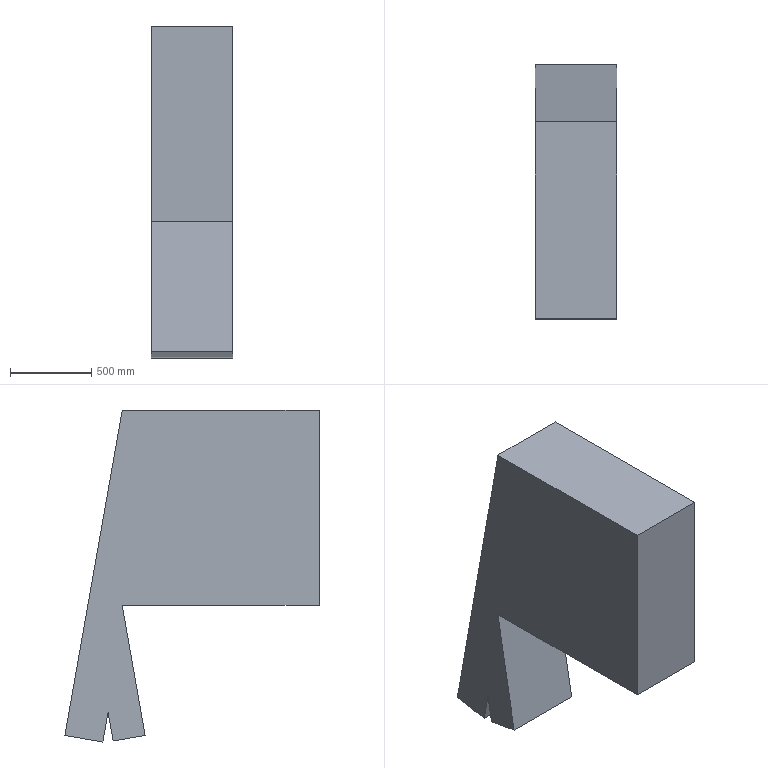Part | STEP file | Material rack | 1 solid | 11 faces | box 500 x 1564 x 2041 mm | volume 933674835 mm3 | plane 11
STEP:
#1=CARTESIAN_POINT('',(0.,0.,0.));
#2=DIRECTION('',(0.,0.,1.));
#3=DIRECTION('',(1.,0.,0.));
#4=AXIS2_PLACEMENT_3D('',#1,#2,#3);
#5=CARTESIAN_POINT('',(250.,1563.716,-800.));
#6=VERTEX_POINT('',#5);
#7=CARTESIAN_POINT('',(250.,1211.062,1200.));
#8=VERTEX_POINT('',#7);
#9=CARTESIAN_POINT('',(250.,1563.716,-800.));
#10=DIRECTION('',(0.,-0.1736,0.9848));
#11=VECTOR('',#10,1.);
#12=LINE('',#9,#11);
#13=CARTESIAN_POINT('',(250.,0.,0.));
#14=DIRECTION('',(1.,0.,0.));
#15=DIRECTION('',(0.,0.,-1.));
#16=AXIS2_PLACEMENT_3D('',#13,#14,#15);
#17=PLANE('',#16);
#18=CARTESIAN_POINT('',(800.,1563.716));
#19=DIRECTION('',(-0.9848,-0.1736));
#20=VECTOR('',#19,1.);
#21=LINE('',#18,#20);
#22=(GEOMETRIC_REPRESENTATION_CONTEXT(2)PARAMETRIC_REPRESENTATION_CONTEXT()REPRESENTATION_CONTEXT('',''));
#23=DEFINITIONAL_REPRESENTATION('',(#21),#22);
#24=PCURVE('',#17,#23);
#25=CARTESIAN_POINT('',(250.,1563.716,-800.));
#26=DIRECTION('',(0.,-0.9848,-0.1736));
#27=DIRECTION('',(0.,0.1736,-0.9848));
#28=AXIS2_PLACEMENT_3D('',#25,#26,#27);
#29=PLANE('',#28);
#30=CARTESIAN_POINT('',(0.,0.));
#31=DIRECTION('',(-1.,0.));
#32=VECTOR('',#31,1.);
#33=LINE('',#30,#32);
#34=(GEOMETRIC_REPRESENTATION_CONTEXT(2)PARAMETRIC_REPRESENTATION_CONTEXT()REPRESENTATION_CONTEXT('',''));
#35=DEFINITIONAL_REPRESENTATION('',(#33),#34);
#36=PCURVE('',#29,#35);
#37=SURFACE_CURVE('',#12,(#24,#36),.PCURVE_S1.);
#38=EDGE_CURVE('',#6,#8,#37,.T.);
#39=ORIENTED_EDGE('',*,*,#38,.T.);
#40=CARTESIAN_POINT('',(250.,0.,1200.));
#41=VERTEX_POINT('',#40);
#42=CARTESIAN_POINT('',(250.,0.,1200.));
#43=DIRECTION('',(0.,-1.,0.));
#44=VECTOR('',#43,1.);
#45=LINE('',#42,#44);
#46=CARTESIAN_POINT('',(-1200.,0.));
#47=DIRECTION('',(0.,-1.));
#48=VECTOR('',#47,1.);
#49=LINE('',#46,#48);
#50=(GEOMETRIC_REPRESENTATION_CONTEXT(2)PARAMETRIC_REPRESENTATION_CONTEXT()REPRESENTATION_CONTEXT('',''));
#51=DEFINITIONAL_REPRESENTATION('',(#49),#50);
#52=PCURVE('',#17,#51);
#53=CARTESIAN_POINT('',(250.,1211.062,1200.));
#54=DIRECTION('',(0.,0.,-1.));
#55=DIRECTION('',(0.,1.,0.));
#56=AXIS2_PLACEMENT_3D('',#53,#54,#55);
#57=PLANE('',#56);
#58=CARTESIAN_POINT('',(-1211.062,0.));
#59=DIRECTION('',(-1.,0.));
#60=VECTOR('',#59,1.);
#61=LINE('',#58,#60);
#62=(GEOMETRIC_REPRESENTATION_CONTEXT(2)PARAMETRIC_REPRESENTATION_CONTEXT()REPRESENTATION_CONTEXT('',''));
#63=DEFINITIONAL_REPRESENTATION('',(#61),#62);
#64=PCURVE('',#57,#63);
#65=SURFACE_CURVE('',#45,(#52,#64),.PCURVE_S1.);
#66=EDGE_CURVE('',#8,#41,#65,.T.);
#67=ORIENTED_EDGE('',*,*,#66,.T.);
#68=CARTESIAN_POINT('',(250.,0.,0.));
#69=VERTEX_POINT('',#68);
#70=CARTESIAN_POINT('',(250.,0.,0.));
#71=DIRECTION('',(0.,0.,-1.));
#72=VECTOR('',#71,1.);
#73=LINE('',#70,#72);
#74=CARTESIAN_POINT('',(0.,0.));
#75=DIRECTION('',(1.,0.));
#76=VECTOR('',#75,1.);
#77=LINE('',#74,#76);
#78=(GEOMETRIC_REPRESENTATION_CONTEXT(2)PARAMETRIC_REPRESENTATION_CONTEXT()REPRESENTATION_CONTEXT('',''));
#79=DEFINITIONAL_REPRESENTATION('',(#77),#78);
#80=PCURVE('',#17,#79);
#81=CARTESIAN_POINT('',(250.,0.,1200.));
#82=DIRECTION('',(0.,1.,0.));
#83=DIRECTION('',(0.,0.,1.));
#84=AXIS2_PLACEMENT_3D('',#81,#82,#83);
#85=PLANE('',#84);
#86=CARTESIAN_POINT('',(-1200.,0.));
#87=DIRECTION('',(-1.,0.));
#88=VECTOR('',#87,1.);
#89=LINE('',#86,#88);
#90=(GEOMETRIC_REPRESENTATION_CONTEXT(2)PARAMETRIC_REPRESENTATION_CONTEXT()REPRESENTATION_CONTEXT('',''));
#91=DEFINITIONAL_REPRESENTATION('',(#89),#90);
#92=PCURVE('',#85,#91);
#93=SURFACE_CURVE('',#73,(#80,#92),.PCURVE_S1.);
#94=EDGE_CURVE('',#41,#69,#93,.T.);
#95=ORIENTED_EDGE('',*,*,#94,.T.);
#96=CARTESIAN_POINT('',(250.,1211.062,0.));
#97=VERTEX_POINT('',#96);
#98=CARTESIAN_POINT('',(250.,0.,0.));
#99=DIRECTION('',(0.,1.,0.));
#100=VECTOR('',#99,1.);
#101=LINE('',#98,#100);
#102=CARTESIAN_POINT('',(0.,0.));
#103=DIRECTION('',(0.,1.));
#104=VECTOR('',#103,1.);
#105=LINE('',#102,#104);
#106=(GEOMETRIC_REPRESENTATION_CONTEXT(2)PARAMETRIC_REPRESENTATION_CONTEXT()REPRESENTATION_CONTEXT('',''));
#107=DEFINITIONAL_REPRESENTATION('',(#105),#106);
#108=PCURVE('',#17,#107);
#109=CARTESIAN_POINT('',(250.,0.,0.));
#110=DIRECTION('',(0.,0.,1.));
#111=DIRECTION('',(0.,-1.,0.));
#112=AXIS2_PLACEMENT_3D('',#109,#110,#111);
#113=PLANE('',#112);
#114=CARTESIAN_POINT('',(0.,0.));
#115=DIRECTION('',(-1.,0.));
#116=VECTOR('',#115,1.);
#117=LINE('',#114,#116);
#118=(GEOMETRIC_REPRESENTATION_CONTEXT(2)PARAMETRIC_REPRESENTATION_CONTEXT()REPRESENTATION_CONTEXT('',''));
#119=DEFINITIONAL_REPRESENTATION('',(#117),#118);
#120=PCURVE('',#113,#119);
#121=SURFACE_CURVE('',#101,(#108,#120),.PCURVE_S1.);
#122=EDGE_CURVE('',#69,#97,#121,.T.);
#123=ORIENTED_EDGE('',*,*,#122,.T.);
#124=CARTESIAN_POINT('',(250.,1070.,-800.));
#125=VERTEX_POINT('',#124);
#126=CARTESIAN_POINT('',(250.,1211.062,0.));
#127=DIRECTION('',(0.,-0.1736,-0.9848));
#128=VECTOR('',#127,1.);
#129=LINE('',#126,#128);
#130=CARTESIAN_POINT('',(0.,1211.062));
#131=DIRECTION('',(0.9848,-0.1736));
#132=VECTOR('',#131,1.);
#133=LINE('',#130,#132);
#134=(GEOMETRIC_REPRESENTATION_CONTEXT(2)PARAMETRIC_REPRESENTATION_CONTEXT()REPRESENTATION_CONTEXT('',''));
#135=DEFINITIONAL_REPRESENTATION('',(#133),#134);
#136=PCURVE('',#17,#135);
#137=CARTESIAN_POINT('',(250.,1211.062,0.));
#138=DIRECTION('',(0.,0.9848,-0.1736));
#139=DIRECTION('',(0.,0.1736,0.9848));
#140=AXIS2_PLACEMENT_3D('',#137,#138,#139);
#141=PLANE('',#140);
#142=CARTESIAN_POINT('',(0.,0.));
#143=DIRECTION('',(-1.,0.));
#144=VECTOR('',#143,1.);
#145=LINE('',#142,#144);
#146=(GEOMETRIC_REPRESENTATION_CONTEXT(2)PARAMETRIC_REPRESENTATION_CONTEXT()REPRESENTATION_CONTEXT('',''));
#147=DEFINITIONAL_REPRESENTATION('',(#145),#146);
#148=PCURVE('',#141,#147);
#149=SURFACE_CURVE('',#129,(#136,#148),.PCURVE_S1.);
#150=EDGE_CURVE('',#97,#125,#149,.T.);
#151=ORIENTED_EDGE('',*,*,#150,.T.);
#152=CARTESIAN_POINT('',(250.,1266.962,-834.73));
#153=VERTEX_POINT('',#152);
#154=CARTESIAN_POINT('',(250.,1070.,-800.));
#155=DIRECTION('',(0.,0.9848,-0.1736));
#156=VECTOR('',#155,1.);
#157=LINE('',#154,#156);
#158=CARTESIAN_POINT('',(800.,1070.));
#159=DIRECTION('',(0.1736,0.9848));
#160=VECTOR('',#159,1.);
#161=LINE('',#158,#160);
#162=(GEOMETRIC_REPRESENTATION_CONTEXT(2)PARAMETRIC_REPRESENTATION_CONTEXT()REPRESENTATION_CONTEXT('',''));
#163=DEFINITIONAL_REPRESENTATION('',(#161),#162);
#164=PCURVE('',#17,#163);
#165=CARTESIAN_POINT('',(250.,1070.,-800.));
#166=DIRECTION('',(0.,0.1736,0.9848));
#167=DIRECTION('',(0.,-0.9848,0.1736));
#168=AXIS2_PLACEMENT_3D('',#165,#166,#167);
#169=PLANE('',#168);
#170=CARTESIAN_POINT('',(0.,0.));
#171=DIRECTION('',(-1.,0.));
#172=VECTOR('',#171,1.);
#173=LINE('',#170,#172);
#174=(GEOMETRIC_REPRESENTATION_CONTEXT(2)PARAMETRIC_REPRESENTATION_CONTEXT()REPRESENTATION_CONTEXT('',''));
#175=DEFINITIONAL_REPRESENTATION('',(#173),#174);
#176=PCURVE('',#169,#175);
#177=SURFACE_CURVE('',#157,(#164,#176),.PCURVE_S1.);
#178=EDGE_CURVE('',#125,#153,#177,.T.);
#179=ORIENTED_EDGE('',*,*,#178,.T.);
#180=CARTESIAN_POINT('',(250.,1297.909,-659.216));
#181=VERTEX_POINT('',#180);
#182=CARTESIAN_POINT('',(250.,1266.962,-834.73));
#183=DIRECTION('',(0.,0.1736,0.9848));
#184=VECTOR('',#183,1.);
#185=LINE('',#182,#184);
#186=CARTESIAN_POINT('',(834.73,1266.962));
#187=DIRECTION('',(-0.9848,0.1736));
#188=VECTOR('',#187,1.);
#189=LINE('',#186,#188);
#190=(GEOMETRIC_REPRESENTATION_CONTEXT(2)PARAMETRIC_REPRESENTATION_CONTEXT()REPRESENTATION_CONTEXT('',''));
#191=DEFINITIONAL_REPRESENTATION('',(#189),#190);
#192=PCURVE('',#17,#191);
#193=CARTESIAN_POINT('',(250.,1266.962,-834.73));
#194=DIRECTION('',(0.,-0.9848,0.1736));
#195=DIRECTION('',(0.,-0.1736,-0.9848));
#196=AXIS2_PLACEMENT_3D('',#193,#194,#195);
#197=PLANE('',#196);
#198=CARTESIAN_POINT('',(0.,0.));
#199=DIRECTION('',(-1.,0.));
#200=VECTOR('',#199,1.);
#201=LINE('',#198,#200);
#202=(GEOMETRIC_REPRESENTATION_CONTEXT(2)PARAMETRIC_REPRESENTATION_CONTEXT()REPRESENTATION_CONTEXT('',''));
#203=DEFINITIONAL_REPRESENTATION('',(#201),#202);
#204=PCURVE('',#197,#203);
#205=SURFACE_CURVE('',#185,(#192,#204),.PCURVE_S1.);
#206=EDGE_CURVE('',#153,#181,#205,.T.);
#207=ORIENTED_EDGE('',*,*,#206,.T.);
#208=CARTESIAN_POINT('',(250.,1330.,-841.21));
#209=VERTEX_POINT('',#208);
#210=CARTESIAN_POINT('',(250.,1297.909,-659.216));
#211=DIRECTION('',(0.,0.1736,-0.9848));
#212=VECTOR('',#211,1.);
#213=LINE('',#210,#212);
#214=CARTESIAN_POINT('',(659.216,1297.909));
#215=DIRECTION('',(0.9848,0.1736));
#216=VECTOR('',#215,1.);
#217=LINE('',#214,#216);
#218=(GEOMETRIC_REPRESENTATION_CONTEXT(2)PARAMETRIC_REPRESENTATION_CONTEXT()REPRESENTATION_CONTEXT('',''));
#219=DEFINITIONAL_REPRESENTATION('',(#217),#218);
#220=PCURVE('',#17,#219);
#221=CARTESIAN_POINT('',(250.,1297.909,-659.216));
#222=DIRECTION('',(0.,0.9848,0.1736));
#223=DIRECTION('',(0.,-0.1736,0.9848));
#224=AXIS2_PLACEMENT_3D('',#221,#222,#223);
#225=PLANE('',#224);
#226=CARTESIAN_POINT('',(0.,0.));
#227=DIRECTION('',(-1.,0.));
#228=VECTOR('',#227,1.);
#229=LINE('',#226,#228);
#230=(GEOMETRIC_REPRESENTATION_CONTEXT(2)PARAMETRIC_REPRESENTATION_CONTEXT()REPRESENTATION_CONTEXT('',''));
#231=DEFINITIONAL_REPRESENTATION('',(#229),#230);
#232=PCURVE('',#225,#231);
#233=SURFACE_CURVE('',#213,(#220,#232),.PCURVE_S1.);
#234=EDGE_CURVE('',#181,#209,#233,.T.);
#235=ORIENTED_EDGE('',*,*,#234,.T.);
#236=CARTESIAN_POINT('',(250.,1330.,-841.21));
#237=DIRECTION('',(0.,0.9848,0.1736));
#238=VECTOR('',#237,1.);
#239=LINE('',#236,#238);
#240=CARTESIAN_POINT('',(841.21,1330.));
#241=DIRECTION('',(-0.1736,0.9848));
#242=VECTOR('',#241,1.);
#243=LINE('',#240,#242);
#244=(GEOMETRIC_REPRESENTATION_CONTEXT(2)PARAMETRIC_REPRESENTATION_CONTEXT()REPRESENTATION_CONTEXT('',''));
#245=DEFINITIONAL_REPRESENTATION('',(#243),#244);
#246=PCURVE('',#17,#245);
#247=CARTESIAN_POINT('',(250.,1330.,-841.21));
#248=DIRECTION('',(0.,-0.1736,0.9848));
#249=DIRECTION('',(0.,-0.9848,-0.1736));
#250=AXIS2_PLACEMENT_3D('',#247,#248,#249);
#251=PLANE('',#250);
#252=CARTESIAN_POINT('',(0.,0.));
#253=DIRECTION('',(-1.,0.));
#254=VECTOR('',#253,1.);
#255=LINE('',#252,#254);
#256=(GEOMETRIC_REPRESENTATION_CONTEXT(2)PARAMETRIC_REPRESENTATION_CONTEXT()REPRESENTATION_CONTEXT('',''));
#257=DEFINITIONAL_REPRESENTATION('',(#255),#256);
#258=PCURVE('',#251,#257);
#259=SURFACE_CURVE('',#239,(#246,#258),.PCURVE_S1.);
#260=EDGE_CURVE('',#209,#6,#259,.T.);
#261=ORIENTED_EDGE('',*,*,#260,.T.);
#262=EDGE_LOOP('',(#39,#67,#95,#123,#151,#179,#207,#235,#261));
#263=FACE_BOUND('',#262,.T.);
#264=ADVANCED_FACE('',(#263),#17,.T.);
#265=CARTESIAN_POINT('',(-250.,0.,1200.));
#266=VERTEX_POINT('',#265);
#267=CARTESIAN_POINT('',(250.,0.,1200.));
#268=DIRECTION('',(-1.,0.,0.));
#269=VECTOR('',#268,1.);
#270=LINE('',#267,#269);
#271=CARTESIAN_POINT('',(-1211.062,0.));
#272=DIRECTION('',(0.,-1.));
#273=VECTOR('',#272,1.);
#274=LINE('',#271,#273);
#275=(GEOMETRIC_REPRESENTATION_CONTEXT(2)PARAMETRIC_REPRESENTATION_CONTEXT()REPRESENTATION_CONTEXT('',''));
#276=DEFINITIONAL_REPRESENTATION('',(#274),#275);
#277=PCURVE('',#57,#276);
#278=CARTESIAN_POINT('',(0.,0.));
#279=DIRECTION('',(0.,-1.));
#280=VECTOR('',#279,1.);
#281=LINE('',#278,#280);
#282=(GEOMETRIC_REPRESENTATION_CONTEXT(2)PARAMETRIC_REPRESENTATION_CONTEXT()REPRESENTATION_CONTEXT('',''));
#283=DEFINITIONAL_REPRESENTATION('',(#281),#282);
#284=PCURVE('',#85,#283);
#285=SURFACE_CURVE('',#270,(#277,#284),.PCURVE_S1.);
#286=EDGE_CURVE('',#41,#266,#285,.T.);
#287=ORIENTED_EDGE('',*,*,#286,.F.);
#288=ORIENTED_EDGE('',*,*,#66,.F.);
#289=CARTESIAN_POINT('',(-250.,1211.062,1200.));
#290=VERTEX_POINT('',#289);
#291=CARTESIAN_POINT('',(250.,1211.062,1200.));
#292=DIRECTION('',(1.,0.,0.));
#293=VECTOR('',#292,1.);
#294=LINE('',#291,#293);
#295=CARTESIAN_POINT('',(0.,0.));
#296=DIRECTION('',(0.,1.));
#297=VECTOR('',#296,1.);
#298=LINE('',#295,#297);
#299=(GEOMETRIC_REPRESENTATION_CONTEXT(2)PARAMETRIC_REPRESENTATION_CONTEXT()REPRESENTATION_CONTEXT('',''));
#300=DEFINITIONAL_REPRESENTATION('',(#298),#299);
#301=PCURVE('',#57,#300);
#302=CARTESIAN_POINT('',(-2030.853,0.));
#303=DIRECTION('',(0.,1.));
#304=VECTOR('',#303,1.);
#305=LINE('',#302,#304);
#306=(GEOMETRIC_REPRESENTATION_CONTEXT(2)PARAMETRIC_REPRESENTATION_CONTEXT()REPRESENTATION_CONTEXT('',''));
#307=DEFINITIONAL_REPRESENTATION('',(#305),#306);
#308=PCURVE('',#29,#307);
#309=SURFACE_CURVE('',#294,(#301,#308),.PCURVE_S1.);
#310=EDGE_CURVE('',#290,#8,#309,.T.);
#311=ORIENTED_EDGE('',*,*,#310,.F.);
#312=CARTESIAN_POINT('',(-250.,1211.062,1200.));
#313=DIRECTION('',(0.,1.,0.));
#314=VECTOR('',#313,1.);
#315=LINE('',#312,#314);
#316=CARTESIAN_POINT('',(0.,-500.));
#317=DIRECTION('',(1.,0.));
#318=VECTOR('',#317,1.);
#319=LINE('',#316,#318);
#320=(GEOMETRIC_REPRESENTATION_CONTEXT(2)PARAMETRIC_REPRESENTATION_CONTEXT()REPRESENTATION_CONTEXT('',''));
#321=DEFINITIONAL_REPRESENTATION('',(#319),#320);
#322=PCURVE('',#57,#321);
#323=CARTESIAN_POINT('',(-250.,0.,0.));
#324=DIRECTION('',(1.,0.,0.));
#325=DIRECTION('',(0.,0.,-1.));
#326=AXIS2_PLACEMENT_3D('',#323,#324,#325);
#327=PLANE('',#326);
#328=CARTESIAN_POINT('',(-1200.,1211.062));
#329=DIRECTION('',(0.,1.));
#330=VECTOR('',#329,1.);
#331=LINE('',#328,#330);
#332=(GEOMETRIC_REPRESENTATION_CONTEXT(2)PARAMETRIC_REPRESENTATION_CONTEXT()REPRESENTATION_CONTEXT('',''));
#333=DEFINITIONAL_REPRESENTATION('',(#331),#332);
#334=PCURVE('',#327,#333);
#335=SURFACE_CURVE('',#315,(#322,#334),.PCURVE_S1.);
#336=EDGE_CURVE('',#266,#290,#335,.T.);
#337=ORIENTED_EDGE('',*,*,#336,.F.);
#338=EDGE_LOOP('',(#287,#288,#311,#337));
#339=FACE_BOUND('',#338,.T.);
#340=ADVANCED_FACE('',(#339),#57,.F.);
#341=ORIENTED_EDGE('',*,*,#310,.T.);
#342=ORIENTED_EDGE('',*,*,#38,.F.);
#343=CARTESIAN_POINT('',(-250.,1563.716,-800.));
#344=VERTEX_POINT('',#343);
#345=CARTESIAN_POINT('',(250.,1563.716,-800.));
#346=DIRECTION('',(1.,0.,0.));
#347=VECTOR('',#346,1.);
#348=LINE('',#345,#347);
#349=CARTESIAN_POINT('',(0.,0.));
#350=DIRECTION('',(0.,1.));
#351=VECTOR('',#350,1.);
#352=LINE('',#349,#351);
#353=(GEOMETRIC_REPRESENTATION_CONTEXT(2)PARAMETRIC_REPRESENTATION_CONTEXT()REPRESENTATION_CONTEXT('',''));
#354=DEFINITIONAL_REPRESENTATION('',(#352),#353);
#355=PCURVE('',#29,#354);
#356=CARTESIAN_POINT('',(-237.321,0.));
#357=DIRECTION('',(0.,1.));
#358=VECTOR('',#357,1.);
#359=LINE('',#356,#358);
#360=(GEOMETRIC_REPRESENTATION_CONTEXT(2)PARAMETRIC_REPRESENTATION_CONTEXT()REPRESENTATION_CONTEXT('',''));
#361=DEFINITIONAL_REPRESENTATION('',(#359),#360);
#362=PCURVE('',#251,#361);
#363=SURFACE_CURVE('',#348,(#355,#362),.PCURVE_S1.);
#364=EDGE_CURVE('',#344,#6,#363,.T.);
#365=ORIENTED_EDGE('',*,*,#364,.F.);
#366=CARTESIAN_POINT('',(-250.,1563.716,-800.));
#367=DIRECTION('',(0.,0.1736,-0.9848));
#368=VECTOR('',#367,1.);
#369=LINE('',#366,#368);
#370=CARTESIAN_POINT('',(0.,-500.));
#371=DIRECTION('',(1.,0.));
#372=VECTOR('',#371,1.);
#373=LINE('',#370,#372);
#374=(GEOMETRIC_REPRESENTATION_CONTEXT(2)PARAMETRIC_REPRESENTATION_CONTEXT()REPRESENTATION_CONTEXT('',''));
#375=DEFINITIONAL_REPRESENTATION('',(#373),#374);
#376=PCURVE('',#29,#375);
#377=CARTESIAN_POINT('',(800.,1563.716));
#378=DIRECTION('',(0.9848,0.1736));
#379=VECTOR('',#378,1.);
#380=LINE('',#377,#379);
#381=(GEOMETRIC_REPRESENTATION_CONTEXT(2)PARAMETRIC_REPRESENTATION_CONTEXT()REPRESENTATION_CONTEXT('',''));
#382=DEFINITIONAL_REPRESENTATION('',(#380),#381);
#383=PCURVE('',#327,#382);
#384=SURFACE_CURVE('',#369,(#376,#383),.PCURVE_S1.);
#385=EDGE_CURVE('',#290,#344,#384,.T.);
#386=ORIENTED_EDGE('',*,*,#385,.F.);
#387=EDGE_LOOP('',(#341,#342,#365,#386));
#388=FACE_BOUND('',#387,.T.);
#389=ADVANCED_FACE('',(#388),#29,.F.);
#390=ORIENTED_EDGE('',*,*,#364,.T.);
#391=ORIENTED_EDGE('',*,*,#260,.F.);
#392=CARTESIAN_POINT('',(-250.,1330.,-841.21));
#393=VERTEX_POINT('',#392);
#394=CARTESIAN_POINT('',(250.,1330.,-841.21));
#395=DIRECTION('',(1.,0.,0.));
#396=VECTOR('',#395,1.);
#397=LINE('',#394,#396);
#398=CARTESIAN_POINT('',(0.,0.));
#399=DIRECTION('',(0.,1.));
#400=VECTOR('',#399,1.);
#401=LINE('',#398,#400);
#402=(GEOMETRIC_REPRESENTATION_CONTEXT(2)PARAMETRIC_REPRESENTATION_CONTEXT()REPRESENTATION_CONTEXT('',''));
#403=DEFINITIONAL_REPRESENTATION('',(#401),#402);
#404=PCURVE('',#251,#403);
#405=CARTESIAN_POINT('',(-184.802,0.));
#406=DIRECTION('',(0.,1.));
#407=VECTOR('',#406,1.);
#408=LINE('',#405,#407);
#409=(GEOMETRIC_REPRESENTATION_CONTEXT(2)PARAMETRIC_REPRESENTATION_CONTEXT()REPRESENTATION_CONTEXT('',''));
#410=DEFINITIONAL_REPRESENTATION('',(#408),#409);
#411=PCURVE('',#225,#410);
#412=SURFACE_CURVE('',#397,(#404,#411),.PCURVE_S1.);
#413=EDGE_CURVE('',#393,#209,#412,.T.);
#414=ORIENTED_EDGE('',*,*,#413,.F.);
#415=CARTESIAN_POINT('',(-250.,1330.,-841.21));
#416=DIRECTION('',(0.,-0.9848,-0.1736));
#417=VECTOR('',#416,1.);
#418=LINE('',#415,#417);
#419=CARTESIAN_POINT('',(0.,-500.));
#420=DIRECTION('',(1.,0.));
#421=VECTOR('',#420,1.);
#422=LINE('',#419,#421);
#423=(GEOMETRIC_REPRESENTATION_CONTEXT(2)PARAMETRIC_REPRESENTATION_CONTEXT()REPRESENTATION_CONTEXT('',''));
#424=DEFINITIONAL_REPRESENTATION('',(#422),#423);
#425=PCURVE('',#251,#424);
#426=CARTESIAN_POINT('',(841.21,1330.));
#427=DIRECTION('',(0.1736,-0.9848));
#428=VECTOR('',#427,1.);
#429=LINE('',#426,#428);
#430=(GEOMETRIC_REPRESENTATION_CONTEXT(2)PARAMETRIC_REPRESENTATION_CONTEXT()REPRESENTATION_CONTEXT('',''));
#431=DEFINITIONAL_REPRESENTATION('',(#429),#430);
#432=PCURVE('',#327,#431);
#433=SURFACE_CURVE('',#418,(#425,#432),.PCURVE_S1.);
#434=EDGE_CURVE('',#344,#393,#433,.T.);
#435=ORIENTED_EDGE('',*,*,#434,.F.);
#436=EDGE_LOOP('',(#390,#391,#414,#435));
#437=FACE_BOUND('',#436,.T.);
#438=ADVANCED_FACE('',(#437),#251,.F.);
#439=ORIENTED_EDGE('',*,*,#413,.T.);
#440=ORIENTED_EDGE('',*,*,#234,.F.);
#441=CARTESIAN_POINT('',(-250.,1297.909,-659.216));
#442=VERTEX_POINT('',#441);
#443=CARTESIAN_POINT('',(250.,1297.909,-659.216));
#444=DIRECTION('',(1.,0.,0.));
#445=VECTOR('',#444,1.);
#446=LINE('',#443,#445);
#447=CARTESIAN_POINT('',(0.,0.));
#448=DIRECTION('',(0.,1.));
#449=VECTOR('',#448,1.);
#450=LINE('',#447,#449);
#451=(GEOMETRIC_REPRESENTATION_CONTEXT(2)PARAMETRIC_REPRESENTATION_CONTEXT()REPRESENTATION_CONTEXT('',''));
#452=DEFINITIONAL_REPRESENTATION('',(#450),#451);
#453=PCURVE('',#225,#452);
#454=CARTESIAN_POINT('',(-178.222,0.));
#455=DIRECTION('',(0.,1.));
#456=VECTOR('',#455,1.);
#457=LINE('',#454,#456);
#458=(GEOMETRIC_REPRESENTATION_CONTEXT(2)PARAMETRIC_REPRESENTATION_CONTEXT()REPRESENTATION_CONTEXT('',''));
#459=DEFINITIONAL_REPRESENTATION('',(#457),#458);
#460=PCURVE('',#197,#459);
#461=SURFACE_CURVE('',#446,(#453,#460),.PCURVE_S1.);
#462=EDGE_CURVE('',#442,#181,#461,.T.);
#463=ORIENTED_EDGE('',*,*,#462,.F.);
#464=CARTESIAN_POINT('',(-250.,1297.909,-659.216));
#465=DIRECTION('',(0.,-0.1736,0.9848));
#466=VECTOR('',#465,1.);
#467=LINE('',#464,#466);
#468=CARTESIAN_POINT('',(0.,-500.));
#469=DIRECTION('',(1.,0.));
#470=VECTOR('',#469,1.);
#471=LINE('',#468,#470);
#472=(GEOMETRIC_REPRESENTATION_CONTEXT(2)PARAMETRIC_REPRESENTATION_CONTEXT()REPRESENTATION_CONTEXT('',''));
#473=DEFINITIONAL_REPRESENTATION('',(#471),#472);
#474=PCURVE('',#225,#473);
#475=CARTESIAN_POINT('',(659.216,1297.909));
#476=DIRECTION('',(-0.9848,-0.1736));
#477=VECTOR('',#476,1.);
#478=LINE('',#475,#477);
#479=(GEOMETRIC_REPRESENTATION_CONTEXT(2)PARAMETRIC_REPRESENTATION_CONTEXT()REPRESENTATION_CONTEXT('',''));
#480=DEFINITIONAL_REPRESENTATION('',(#478),#479);
#481=PCURVE('',#327,#480);
#482=SURFACE_CURVE('',#467,(#474,#481),.PCURVE_S1.);
#483=EDGE_CURVE('',#393,#442,#482,.T.);
#484=ORIENTED_EDGE('',*,*,#483,.F.);
#485=EDGE_LOOP('',(#439,#440,#463,#484));
#486=FACE_BOUND('',#485,.T.);
#487=ADVANCED_FACE('',(#486),#225,.F.);
#488=ORIENTED_EDGE('',*,*,#462,.T.);
#489=ORIENTED_EDGE('',*,*,#206,.F.);
#490=CARTESIAN_POINT('',(-250.,1266.962,-834.73));
#491=VERTEX_POINT('',#490);
#492=CARTESIAN_POINT('',(250.,1266.962,-834.73));
#493=DIRECTION('',(1.,0.,0.));
#494=VECTOR('',#493,1.);
#495=LINE('',#492,#494);
#496=CARTESIAN_POINT('',(0.,0.));
#497=DIRECTION('',(0.,1.));
#498=VECTOR('',#497,1.);
#499=LINE('',#496,#498);
#500=(GEOMETRIC_REPRESENTATION_CONTEXT(2)PARAMETRIC_REPRESENTATION_CONTEXT()REPRESENTATION_CONTEXT('',''));
#501=DEFINITIONAL_REPRESENTATION('',(#499),#500);
#502=PCURVE('',#197,#501);
#503=CARTESIAN_POINT('',(-200.,0.));
#504=DIRECTION('',(0.,1.));
#505=VECTOR('',#504,1.);
#506=LINE('',#503,#505);
#507=(GEOMETRIC_REPRESENTATION_CONTEXT(2)PARAMETRIC_REPRESENTATION_CONTEXT()REPRESENTATION_CONTEXT('',''));
#508=DEFINITIONAL_REPRESENTATION('',(#506),#507);
#509=PCURVE('',#169,#508);
#510=SURFACE_CURVE('',#495,(#502,#509),.PCURVE_S1.);
#511=EDGE_CURVE('',#491,#153,#510,.T.);
#512=ORIENTED_EDGE('',*,*,#511,.F.);
#513=CARTESIAN_POINT('',(-250.,1266.962,-834.73));
#514=DIRECTION('',(0.,-0.1736,-0.9848));
#515=VECTOR('',#514,1.);
#516=LINE('',#513,#515);
#517=CARTESIAN_POINT('',(0.,-500.));
#518=DIRECTION('',(1.,0.));
#519=VECTOR('',#518,1.);
#520=LINE('',#517,#519);
#521=(GEOMETRIC_REPRESENTATION_CONTEXT(2)PARAMETRIC_REPRESENTATION_CONTEXT()REPRESENTATION_CONTEXT('',''));
#522=DEFINITIONAL_REPRESENTATION('',(#520),#521);
#523=PCURVE('',#197,#522);
#524=CARTESIAN_POINT('',(834.73,1266.962));
#525=DIRECTION('',(0.9848,-0.1736));
#526=VECTOR('',#525,1.);
#527=LINE('',#524,#526);
#528=(GEOMETRIC_REPRESENTATION_CONTEXT(2)PARAMETRIC_REPRESENTATION_CONTEXT()REPRESENTATION_CONTEXT('',''));
#529=DEFINITIONAL_REPRESENTATION('',(#527),#528);
#530=PCURVE('',#327,#529);
#531=SURFACE_CURVE('',#516,(#523,#530),.PCURVE_S1.);
#532=EDGE_CURVE('',#442,#491,#531,.T.);
#533=ORIENTED_EDGE('',*,*,#532,.F.);
#534=EDGE_LOOP('',(#488,#489,#512,#533));
#535=FACE_BOUND('',#534,.T.);
#536=ADVANCED_FACE('',(#535),#197,.F.);
#537=ORIENTED_EDGE('',*,*,#511,.T.);
#538=ORIENTED_EDGE('',*,*,#178,.F.);
#539=CARTESIAN_POINT('',(-250.,1070.,-800.));
#540=VERTEX_POINT('',#539);
#541=CARTESIAN_POINT('',(250.,1070.,-800.));
#542=DIRECTION('',(1.,0.,0.));
#543=VECTOR('',#542,1.);
#544=LINE('',#541,#543);
#545=CARTESIAN_POINT('',(0.,0.));
#546=DIRECTION('',(0.,1.));
#547=VECTOR('',#546,1.);
#548=LINE('',#545,#547);
#549=(GEOMETRIC_REPRESENTATION_CONTEXT(2)PARAMETRIC_REPRESENTATION_CONTEXT()REPRESENTATION_CONTEXT('',''));
#550=DEFINITIONAL_REPRESENTATION('',(#548),#549);
#551=PCURVE('',#169,#550);
#552=CARTESIAN_POINT('',(-812.341,0.));
#553=DIRECTION('',(0.,1.));
#554=VECTOR('',#553,1.);
#555=LINE('',#552,#554);
#556=(GEOMETRIC_REPRESENTATION_CONTEXT(2)PARAMETRIC_REPRESENTATION_CONTEXT()REPRESENTATION_CONTEXT('',''));
#557=DEFINITIONAL_REPRESENTATION('',(#555),#556);
#558=PCURVE('',#141,#557);
#559=SURFACE_CURVE('',#544,(#551,#558),.PCURVE_S1.);
#560=EDGE_CURVE('',#540,#125,#559,.T.);
#561=ORIENTED_EDGE('',*,*,#560,.F.);
#562=CARTESIAN_POINT('',(-250.,1070.,-800.));
#563=DIRECTION('',(0.,-0.9848,0.1736));
#564=VECTOR('',#563,1.);
#565=LINE('',#562,#564);
#566=CARTESIAN_POINT('',(0.,-500.));
#567=DIRECTION('',(1.,0.));
#568=VECTOR('',#567,1.);
#569=LINE('',#566,#568);
#570=(GEOMETRIC_REPRESENTATION_CONTEXT(2)PARAMETRIC_REPRESENTATION_CONTEXT()REPRESENTATION_CONTEXT('',''));
#571=DEFINITIONAL_REPRESENTATION('',(#569),#570);
#572=PCURVE('',#169,#571);
#573=CARTESIAN_POINT('',(800.,1070.));
#574=DIRECTION('',(-0.1736,-0.9848));
#575=VECTOR('',#574,1.);
#576=LINE('',#573,#575);
#577=(GEOMETRIC_REPRESENTATION_CONTEXT(2)PARAMETRIC_REPRESENTATION_CONTEXT()REPRESENTATION_CONTEXT('',''));
#578=DEFINITIONAL_REPRESENTATION('',(#576),#577);
#579=PCURVE('',#327,#578);
#580=SURFACE_CURVE('',#565,(#572,#579),.PCURVE_S1.);
#581=EDGE_CURVE('',#491,#540,#580,.T.);
#582=ORIENTED_EDGE('',*,*,#581,.F.);
#583=EDGE_LOOP('',(#537,#538,#561,#582));
#584=FACE_BOUND('',#583,.T.);
#585=ADVANCED_FACE('',(#584),#169,.F.);
#586=ORIENTED_EDGE('',*,*,#560,.T.);
#587=ORIENTED_EDGE('',*,*,#150,.F.);
#588=CARTESIAN_POINT('',(-250.,1211.062,0.));
#589=VERTEX_POINT('',#588);
#590=CARTESIAN_POINT('',(250.,1211.062,0.));
#591=DIRECTION('',(1.,0.,0.));
#592=VECTOR('',#591,1.);
#593=LINE('',#590,#592);
#594=CARTESIAN_POINT('',(0.,0.));
#595=DIRECTION('',(0.,1.));
#596=VECTOR('',#595,1.);
#597=LINE('',#594,#596);
#598=(GEOMETRIC_REPRESENTATION_CONTEXT(2)PARAMETRIC_REPRESENTATION_CONTEXT()REPRESENTATION_CONTEXT('',''));
#599=DEFINITIONAL_REPRESENTATION('',(#597),#598);
#600=PCURVE('',#141,#599);
#601=CARTESIAN_POINT('',(-1211.062,0.));
#602=DIRECTION('',(0.,1.));
#603=VECTOR('',#602,1.);
#604=LINE('',#601,#603);
#605=(GEOMETRIC_REPRESENTATION_CONTEXT(2)PARAMETRIC_REPRESENTATION_CONTEXT()REPRESENTATION_CONTEXT('',''));
#606=DEFINITIONAL_REPRESENTATION('',(#604),#605);
#607=PCURVE('',#113,#606);
#608=SURFACE_CURVE('',#593,(#600,#607),.PCURVE_S1.);
#609=EDGE_CURVE('',#589,#97,#608,.T.);
#610=ORIENTED_EDGE('',*,*,#609,.F.);
#611=CARTESIAN_POINT('',(-250.,1211.062,0.));
#612=DIRECTION('',(0.,0.1736,0.9848));
#613=VECTOR('',#612,1.);
#614=LINE('',#611,#613);
#615=CARTESIAN_POINT('',(0.,-500.));
#616=DIRECTION('',(1.,0.));
#617=VECTOR('',#616,1.);
#618=LINE('',#615,#617);
#619=(GEOMETRIC_REPRESENTATION_CONTEXT(2)PARAMETRIC_REPRESENTATION_CONTEXT()REPRESENTATION_CONTEXT('',''));
#620=DEFINITIONAL_REPRESENTATION('',(#618),#619);
#621=PCURVE('',#141,#620);
#622=CARTESIAN_POINT('',(0.,1211.062));
#623=DIRECTION('',(-0.9848,0.1736));
#624=VECTOR('',#623,1.);
#625=LINE('',#622,#624);
#626=(GEOMETRIC_REPRESENTATION_CONTEXT(2)PARAMETRIC_REPRESENTATION_CONTEXT()REPRESENTATION_CONTEXT('',''));
#627=DEFINITIONAL_REPRESENTATION('',(#625),#626);
#628=PCURVE('',#327,#627);
#629=SURFACE_CURVE('',#614,(#621,#628),.PCURVE_S1.);
#630=EDGE_CURVE('',#540,#589,#629,.T.);
#631=ORIENTED_EDGE('',*,*,#630,.F.);
#632=EDGE_LOOP('',(#586,#587,#610,#631));
#633=FACE_BOUND('',#632,.T.);
#634=ADVANCED_FACE('',(#633),#141,.F.);
#635=ORIENTED_EDGE('',*,*,#609,.T.);
#636=ORIENTED_EDGE('',*,*,#122,.F.);
#637=CARTESIAN_POINT('',(-250.,0.,0.));
#638=VERTEX_POINT('',#637);
#639=CARTESIAN_POINT('',(250.,0.,0.));
#640=DIRECTION('',(1.,0.,0.));
#641=VECTOR('',#640,1.);
#642=LINE('',#639,#641);
#643=CARTESIAN_POINT('',(0.,0.));
#644=DIRECTION('',(0.,1.));
#645=VECTOR('',#644,1.);
#646=LINE('',#643,#645);
#647=(GEOMETRIC_REPRESENTATION_CONTEXT(2)PARAMETRIC_REPRESENTATION_CONTEXT()REPRESENTATION_CONTEXT('',''));
#648=DEFINITIONAL_REPRESENTATION('',(#646),#647);
#649=PCURVE('',#113,#648);
#650=CARTESIAN_POINT('',(-1200.,0.));
#651=DIRECTION('',(0.,1.));
#652=VECTOR('',#651,1.);
#653=LINE('',#650,#652);
#654=(GEOMETRIC_REPRESENTATION_CONTEXT(2)PARAMETRIC_REPRESENTATION_CONTEXT()REPRESENTATION_CONTEXT('',''));
#655=DEFINITIONAL_REPRESENTATION('',(#653),#654);
#656=PCURVE('',#85,#655);
#657=SURFACE_CURVE('',#642,(#649,#656),.PCURVE_S1.);
#658=EDGE_CURVE('',#638,#69,#657,.T.);
#659=ORIENTED_EDGE('',*,*,#658,.F.);
#660=CARTESIAN_POINT('',(-250.,0.,0.));
#661=DIRECTION('',(0.,-1.,0.));
#662=VECTOR('',#661,1.);
#663=LINE('',#660,#662);
#664=CARTESIAN_POINT('',(0.,-500.));
#665=DIRECTION('',(1.,0.));
#666=VECTOR('',#665,1.);
#667=LINE('',#664,#666);
#668=(GEOMETRIC_REPRESENTATION_CONTEXT(2)PARAMETRIC_REPRESENTATION_CONTEXT()REPRESENTATION_CONTEXT('',''));
#669=DEFINITIONAL_REPRESENTATION('',(#667),#668);
#670=PCURVE('',#113,#669);
#671=CARTESIAN_POINT('',(0.,0.));
#672=DIRECTION('',(0.,-1.));
#673=VECTOR('',#672,1.);
#674=LINE('',#671,#673);
#675=(GEOMETRIC_REPRESENTATION_CONTEXT(2)PARAMETRIC_REPRESENTATION_CONTEXT()REPRESENTATION_CONTEXT('',''));
#676=DEFINITIONAL_REPRESENTATION('',(#674),#675);
#677=PCURVE('',#327,#676);
#678=SURFACE_CURVE('',#663,(#670,#677),.PCURVE_S1.);
#679=EDGE_CURVE('',#589,#638,#678,.T.);
#680=ORIENTED_EDGE('',*,*,#679,.F.);
#681=EDGE_LOOP('',(#635,#636,#659,#680));
#682=FACE_BOUND('',#681,.T.);
#683=ADVANCED_FACE('',(#682),#113,.F.);
#684=ORIENTED_EDGE('',*,*,#658,.T.);
#685=ORIENTED_EDGE('',*,*,#94,.F.);
#686=ORIENTED_EDGE('',*,*,#286,.T.);
#687=CARTESIAN_POINT('',(-250.,0.,1200.));
#688=DIRECTION('',(0.,0.,1.));
#689=VECTOR('',#688,1.);
#690=LINE('',#687,#689);
#691=CARTESIAN_POINT('',(0.,-500.));
#692=DIRECTION('',(1.,0.));
#693=VECTOR('',#692,1.);
#694=LINE('',#691,#693);
#695=(GEOMETRIC_REPRESENTATION_CONTEXT(2)PARAMETRIC_REPRESENTATION_CONTEXT()REPRESENTATION_CONTEXT('',''));
#696=DEFINITIONAL_REPRESENTATION('',(#694),#695);
#697=PCURVE('',#85,#696);
#698=CARTESIAN_POINT('',(-1200.,0.));
#699=DIRECTION('',(-1.,0.));
#700=VECTOR('',#699,1.);
#701=LINE('',#698,#700);
#702=(GEOMETRIC_REPRESENTATION_CONTEXT(2)PARAMETRIC_REPRESENTATION_CONTEXT()REPRESENTATION_CONTEXT('',''));
#703=DEFINITIONAL_REPRESENTATION('',(#701),#702);
#704=PCURVE('',#327,#703);
#705=SURFACE_CURVE('',#690,(#697,#704),.PCURVE_S1.);
#706=EDGE_CURVE('',#638,#266,#705,.T.);
#707=ORIENTED_EDGE('',*,*,#706,.F.);
#708=EDGE_LOOP('',(#684,#685,#686,#707));
#709=FACE_BOUND('',#708,.T.);
#710=ADVANCED_FACE('',(#709),#85,.F.);
#711=ORIENTED_EDGE('',*,*,#336,.T.);
#712=ORIENTED_EDGE('',*,*,#385,.T.);
#713=ORIENTED_EDGE('',*,*,#434,.T.);
#714=ORIENTED_EDGE('',*,*,#483,.T.);
#715=ORIENTED_EDGE('',*,*,#532,.T.);
#716=ORIENTED_EDGE('',*,*,#581,.T.);
#717=ORIENTED_EDGE('',*,*,#630,.T.);
#718=ORIENTED_EDGE('',*,*,#679,.T.);
#719=ORIENTED_EDGE('',*,*,#706,.T.);
#720=EDGE_LOOP('',(#711,#712,#713,#714,#715,#716,#717,#718,#719));
#721=FACE_BOUND('',#720,.T.);
#722=ADVANCED_FACE('',(#721),#327,.F.);
#723=CLOSED_SHELL('',(#264,#340,#389,#438,#487,#536,#585,#634,#683,#710,#722));
#724=MANIFOLD_SOLID_BREP('',#723);
#725=(LENGTH_UNIT()NAMED_UNIT(*)SI_UNIT(.MILLI.,.METRE.));
#726=UNCERTAINTY_MEASURE_WITH_UNIT(LENGTH_MEASURE(0.0000001),#725,'','');
#727=(NAMED_UNIT(*)PLANE_ANGLE_UNIT()SI_UNIT($,.RADIAN.));
#728=(NAMED_UNIT(*)SI_UNIT($,.STERADIAN.)SOLID_ANGLE_UNIT());
#729=(GEOMETRIC_REPRESENTATION_CONTEXT(3)GLOBAL_UNCERTAINTY_ASSIGNED_CONTEXT((#726))GLOBAL_UNIT_ASSIGNED_CONTEXT((#725,#727,#728))REPRESENTATION_CONTEXT('',''));
#730=ADVANCED_BREP_SHAPE_REPRESENTATION('',(#4,#724),#729);